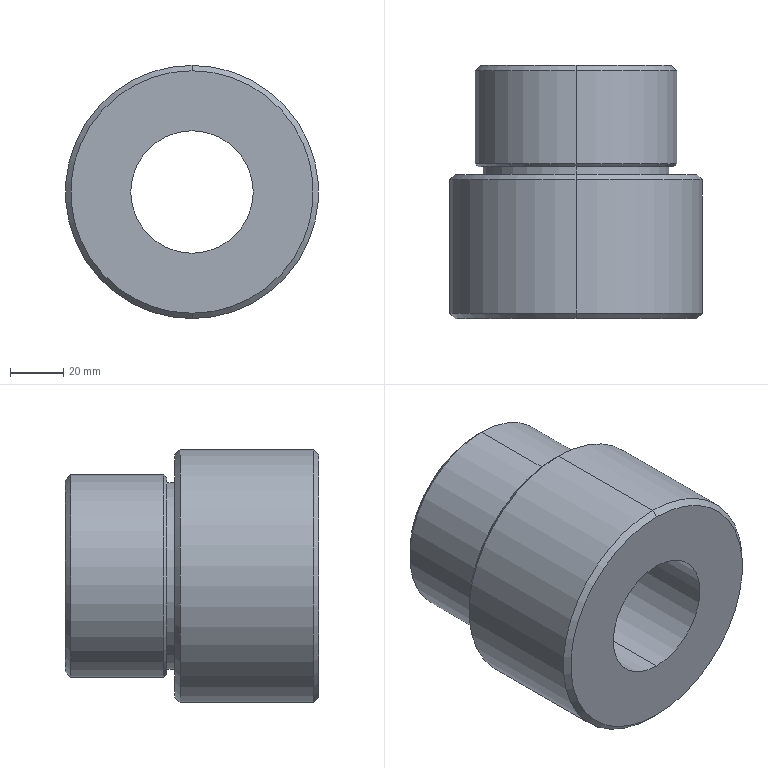Part | SolidWorks | features BaseBody 1 | 1 solid | 20 faces | box 95 x 95 x 95 mm | volume 407029 mm3 | cylinder 8 | cone 8 | plane 4 | commonest cylinder face diameters 46 x2 70 x2 76 x2 95 x2
STEP:
#1=CARTESIAN_POINT('',(0.,0.,-23.));
#2=VERTEX_POINT('',#1);
#3=CARTESIAN_POINT('',(0.,0.,23.));
#4=VERTEX_POINT('',#3);
#5=CARTESIAN_POINT('',(0.,0.,0.));
#6=DIRECTION('',(0.,1.,0.));
#7=DIRECTION('',(0.,0.,1.));
#8=AXIS2_PLACEMENT_3D('',#5,#6,#7);
#9=CIRCLE('',#8,23.);
#10=EDGE_CURVE('',#2,#4,#9,.T.);
#11=ORIENTED_EDGE('',*,*,#10,.F.);
#12=CARTESIAN_POINT('',(0.,95.,-23.));
#13=VERTEX_POINT('',#12);
#14=CARTESIAN_POINT('',(0.,95.,-23.));
#15=DIRECTION('',(0.,1.,0.));
#16=VECTOR('',#15,1000.);
#17=LINE('',#14,#16);
#18=EDGE_CURVE('',#2,#13,#17,.T.);
#19=ORIENTED_EDGE('',*,*,#18,.T.);
#20=CARTESIAN_POINT('',(0.,95.,23.));
#21=VERTEX_POINT('',#20);
#22=CARTESIAN_POINT('',(0.,95.,0.));
#23=DIRECTION('',(0.,1.,0.));
#24=DIRECTION('',(0.,0.,1.));
#25=AXIS2_PLACEMENT_3D('',#22,#23,#24);
#26=CIRCLE('',#25,23.);
#27=EDGE_CURVE('',#13,#21,#26,.T.);
#28=ORIENTED_EDGE('',*,*,#27,.T.);
#29=CARTESIAN_POINT('',(0.,95.,23.));
#30=DIRECTION('',(0.,1.,0.));
#31=VECTOR('',#30,1000.);
#32=LINE('',#29,#31);
#33=EDGE_CURVE('',#4,#21,#32,.T.);
#34=ORIENTED_EDGE('',*,*,#33,.F.);
#35=EDGE_LOOP('',(#11,#19,#28,#34));
#36=FACE_OUTER_BOUND('',#35,.T.);
#37=CARTESIAN_POINT('',(0.,95.,0.));
#38=DIRECTION('',(0.,1.,0.));
#39=DIRECTION('',(0.,0.,1.));
#40=AXIS2_PLACEMENT_3D('',#37,#38,#39);
#41=CYLINDRICAL_SURFACE('',#40,23.);
#42=ADVANCED_FACE('',(#36),#41,.F.);
#43=CARTESIAN_POINT('',(0.,93.,-38.));
#44=VERTEX_POINT('',#43);
#45=CARTESIAN_POINT('',(0.,93.,38.));
#46=VERTEX_POINT('',#45);
#47=CARTESIAN_POINT('',(0.,93.,0.));
#48=DIRECTION('',(0.,-1.,0.));
#49=DIRECTION('',(0.,0.,1.));
#50=AXIS2_PLACEMENT_3D('',#47,#48,#49);
#51=CIRCLE('',#50,38.);
#52=EDGE_CURVE('',#44,#46,#51,.T.);
#53=ORIENTED_EDGE('',*,*,#52,.T.);
#54=CARTESIAN_POINT('',(0.,58.083,38.));
#55=VERTEX_POINT('',#54);
#56=CARTESIAN_POINT('',(0.,95.,38.));
#57=DIRECTION('',(0.,-1.,0.));
#58=VECTOR('',#57,1000.);
#59=LINE('',#56,#58);
#60=EDGE_CURVE('',#46,#55,#59,.T.);
#61=ORIENTED_EDGE('',*,*,#60,.T.);
#62=CARTESIAN_POINT('',(0.,58.083,-38.));
#63=VERTEX_POINT('',#62);
#64=CARTESIAN_POINT('',(0.,58.083,0.));
#65=DIRECTION('',(0.,1.,0.));
#66=DIRECTION('',(0.,0.,1.));
#67=AXIS2_PLACEMENT_3D('',#64,#65,#66);
#68=CIRCLE('',#67,38.);
#69=EDGE_CURVE('',#55,#63,#68,.T.);
#70=ORIENTED_EDGE('',*,*,#69,.T.);
#71=CARTESIAN_POINT('',(0.,95.,-38.));
#72=DIRECTION('',(0.,-1.,0.));
#73=VECTOR('',#72,1000.);
#74=LINE('',#71,#73);
#75=EDGE_CURVE('',#44,#63,#74,.T.);
#76=ORIENTED_EDGE('',*,*,#75,.F.);
#77=EDGE_LOOP('',(#53,#61,#70,#76));
#78=FACE_OUTER_BOUND('',#77,.T.);
#79=CARTESIAN_POINT('',(0.,95.,0.));
#80=DIRECTION('',(0.,-1.,0.));
#81=DIRECTION('',(0.,0.,-1.));
#82=AXIS2_PLACEMENT_3D('',#79,#80,#81);
#83=CYLINDRICAL_SURFACE('',#82,38.);
#84=ADVANCED_FACE('',(#78),#83,.T.);
#85=CARTESIAN_POINT('',(0.,95.,36.));
#86=VERTEX_POINT('',#85);
#87=CARTESIAN_POINT('',(0.,95.,-36.));
#88=VERTEX_POINT('',#87);
#89=CARTESIAN_POINT('',(0.,95.,0.));
#90=DIRECTION('',(0.,1.,0.));
#91=DIRECTION('',(0.,0.,1.));
#92=AXIS2_PLACEMENT_3D('',#89,#90,#91);
#93=CIRCLE('',#92,36.);
#94=EDGE_CURVE('',#86,#88,#93,.T.);
#95=ORIENTED_EDGE('',*,*,#94,.F.);
#96=CARTESIAN_POINT('',(0.,95.,36.));
#97=DIRECTION('',(0.,-0.7071,0.7071));
#98=VECTOR('',#97,1000.);
#99=LINE('',#96,#98);
#100=EDGE_CURVE('',#86,#46,#99,.T.);
#101=ORIENTED_EDGE('',*,*,#100,.T.);
#102=ORIENTED_EDGE('',*,*,#52,.F.);
#103=CARTESIAN_POINT('',(0.,95.,-36.));
#104=DIRECTION('',(0.,-0.7071,-0.7071));
#105=VECTOR('',#104,1000.);
#106=LINE('',#103,#105);
#107=EDGE_CURVE('',#88,#44,#106,.T.);
#108=ORIENTED_EDGE('',*,*,#107,.F.);
#109=EDGE_LOOP('',(#95,#101,#102,#108));
#110=FACE_OUTER_BOUND('',#109,.T.);
#111=CARTESIAN_POINT('',(0.,95.,0.));
#112=DIRECTION('',(0.,-1.,0.));
#113=DIRECTION('',(0.,0.,-1.));
#114=AXIS2_PLACEMENT_3D('',#111,#112,#113);
#115=CONICAL_SURFACE('',#114,36.,0.7854);
#116=ADVANCED_FACE('',(#110),#115,.T.);
#117=CARTESIAN_POINT('',(0.,57.,36.917));
#118=VERTEX_POINT('',#117);
#119=CARTESIAN_POINT('',(0.,57.,-36.917));
#120=VERTEX_POINT('',#119);
#121=CARTESIAN_POINT('',(0.,57.,0.));
#122=DIRECTION('',(0.,1.,0.));
#123=DIRECTION('',(0.,0.,1.));
#124=AXIS2_PLACEMENT_3D('',#121,#122,#123);
#125=CIRCLE('',#124,36.917);
#126=EDGE_CURVE('',#118,#120,#125,.T.);
#127=ORIENTED_EDGE('',*,*,#126,.T.);
#128=CARTESIAN_POINT('',(0.,57.,-36.917));
#129=DIRECTION('',(0.,0.7071,-0.7071));
#130=VECTOR('',#129,1000.);
#131=LINE('',#128,#130);
#132=EDGE_CURVE('',#120,#63,#131,.T.);
#133=ORIENTED_EDGE('',*,*,#132,.T.);
#134=ORIENTED_EDGE('',*,*,#69,.F.);
#135=CARTESIAN_POINT('',(0.,57.,36.917));
#136=DIRECTION('',(0.,0.7071,0.7071));
#137=VECTOR('',#136,1000.);
#138=LINE('',#135,#137);
#139=EDGE_CURVE('',#118,#55,#138,.T.);
#140=ORIENTED_EDGE('',*,*,#139,.F.);
#141=EDGE_LOOP('',(#127,#133,#134,#140));
#142=FACE_OUTER_BOUND('',#141,.T.);
#143=CARTESIAN_POINT('',(0.,57.,0.));
#144=DIRECTION('',(0.,1.,0.));
#145=DIRECTION('',(0.,0.,1.));
#146=AXIS2_PLACEMENT_3D('',#143,#144,#145);
#147=CONICAL_SURFACE('',#146,36.917,0.7854);
#148=ADVANCED_FACE('',(#142),#147,.T.);
#149=CARTESIAN_POINT('',(0.,54.,45.5));
#150=VERTEX_POINT('',#149);
#151=CARTESIAN_POINT('',(0.,54.,-45.5));
#152=VERTEX_POINT('',#151);
#153=CARTESIAN_POINT('',(0.,54.,0.));
#154=DIRECTION('',(0.,1.,0.));
#155=DIRECTION('',(0.,0.,1.));
#156=AXIS2_PLACEMENT_3D('',#153,#154,#155);
#157=CIRCLE('',#156,45.5);
#158=EDGE_CURVE('',#150,#152,#157,.T.);
#159=ORIENTED_EDGE('',*,*,#158,.F.);
#160=CARTESIAN_POINT('',(0.,52.,47.5));
#161=VERTEX_POINT('',#160);
#162=CARTESIAN_POINT('',(0.,54.,45.5));
#163=DIRECTION('',(0.,-0.7071,0.7071));
#164=VECTOR('',#163,1000.);
#165=LINE('',#162,#164);
#166=EDGE_CURVE('',#150,#161,#165,.T.);
#167=ORIENTED_EDGE('',*,*,#166,.T.);
#168=CARTESIAN_POINT('',(0.,52.,-47.5));
#169=VERTEX_POINT('',#168);
#170=CARTESIAN_POINT('',(0.,52.,0.));
#171=DIRECTION('',(0.,-1.,0.));
#172=DIRECTION('',(0.,0.,1.));
#173=AXIS2_PLACEMENT_3D('',#170,#171,#172);
#174=CIRCLE('',#173,47.5);
#175=EDGE_CURVE('',#169,#161,#174,.T.);
#176=ORIENTED_EDGE('',*,*,#175,.F.);
#177=CARTESIAN_POINT('',(0.,54.,-45.5));
#178=DIRECTION('',(0.,-0.7071,-0.7071));
#179=VECTOR('',#178,1000.);
#180=LINE('',#177,#179);
#181=EDGE_CURVE('',#152,#169,#180,.T.);
#182=ORIENTED_EDGE('',*,*,#181,.F.);
#183=EDGE_LOOP('',(#159,#167,#176,#182));
#184=FACE_OUTER_BOUND('',#183,.T.);
#185=CARTESIAN_POINT('',(0.,54.,0.));
#186=DIRECTION('',(0.,-1.,0.));
#187=DIRECTION('',(0.,0.,-1.));
#188=AXIS2_PLACEMENT_3D('',#185,#186,#187);
#189=CONICAL_SURFACE('',#188,45.5,0.7854);
#190=ADVANCED_FACE('',(#184),#189,.T.);
#191=CARTESIAN_POINT('',(0.,0.,-45.5));
#192=VERTEX_POINT('',#191);
#193=CARTESIAN_POINT('',(0.,0.,45.5));
#194=VERTEX_POINT('',#193);
#195=CARTESIAN_POINT('',(0.,0.,0.));
#196=DIRECTION('',(0.,-1.,0.));
#197=DIRECTION('',(0.,0.,1.));
#198=AXIS2_PLACEMENT_3D('',#195,#196,#197);
#199=CIRCLE('',#198,45.5);
#200=EDGE_CURVE('',#192,#194,#199,.T.);
#201=ORIENTED_EDGE('',*,*,#200,.F.);
#202=CARTESIAN_POINT('',(0.,2.,-47.5));
#203=VERTEX_POINT('',#202);
#204=CARTESIAN_POINT('',(0.,2.,-47.5));
#205=DIRECTION('',(0.,0.7071,-0.7071));
#206=VECTOR('',#205,1000.);
#207=LINE('',#204,#206);
#208=EDGE_CURVE('',#192,#203,#207,.T.);
#209=ORIENTED_EDGE('',*,*,#208,.T.);
#210=CARTESIAN_POINT('',(0.,2.,47.5));
#211=VERTEX_POINT('',#210);
#212=CARTESIAN_POINT('',(0.,2.,0.));
#213=DIRECTION('',(0.,1.,0.));
#214=DIRECTION('',(0.,0.,1.));
#215=AXIS2_PLACEMENT_3D('',#212,#213,#214);
#216=CIRCLE('',#215,47.5);
#217=EDGE_CURVE('',#211,#203,#216,.T.);
#218=ORIENTED_EDGE('',*,*,#217,.F.);
#219=CARTESIAN_POINT('',(0.,2.,47.5));
#220=DIRECTION('',(0.,0.7071,0.7071));
#221=VECTOR('',#220,1000.);
#222=LINE('',#219,#221);
#223=EDGE_CURVE('',#194,#211,#222,.T.);
#224=ORIENTED_EDGE('',*,*,#223,.F.);
#225=EDGE_LOOP('',(#201,#209,#218,#224));
#226=FACE_OUTER_BOUND('',#225,.T.);
#227=CARTESIAN_POINT('',(0.,2.,0.));
#228=DIRECTION('',(0.,1.,0.));
#229=DIRECTION('',(0.,0.,1.));
#230=AXIS2_PLACEMENT_3D('',#227,#228,#229);
#231=CONICAL_SURFACE('',#230,47.5,0.7854);
#232=ADVANCED_FACE('',(#226),#231,.T.);
#233=CARTESIAN_POINT('',(0.,57.,35.));
#234=VERTEX_POINT('',#233);
#235=CARTESIAN_POINT('',(0.,57.,-35.));
#236=VERTEX_POINT('',#235);
#237=CARTESIAN_POINT('',(0.,57.,0.));
#238=DIRECTION('',(0.,1.,0.));
#239=DIRECTION('',(0.,0.,1.));
#240=AXIS2_PLACEMENT_3D('',#237,#238,#239);
#241=CIRCLE('',#240,35.);
#242=EDGE_CURVE('',#234,#236,#241,.T.);
#243=ORIENTED_EDGE('',*,*,#242,.F.);
#244=CARTESIAN_POINT('',(0.,54.,35.));
#245=VERTEX_POINT('',#244);
#246=CARTESIAN_POINT('',(0.,57.,35.));
#247=DIRECTION('',(0.,-1.,0.));
#248=VECTOR('',#247,1000.);
#249=LINE('',#246,#248);
#250=EDGE_CURVE('',#234,#245,#249,.T.);
#251=ORIENTED_EDGE('',*,*,#250,.T.);
#252=CARTESIAN_POINT('',(0.,54.,-35.));
#253=VERTEX_POINT('',#252);
#254=CARTESIAN_POINT('',(0.,54.,0.));
#255=DIRECTION('',(0.,1.,0.));
#256=DIRECTION('',(0.,0.,1.));
#257=AXIS2_PLACEMENT_3D('',#254,#255,#256);
#258=CIRCLE('',#257,35.);
#259=EDGE_CURVE('',#245,#253,#258,.T.);
#260=ORIENTED_EDGE('',*,*,#259,.T.);
#261=CARTESIAN_POINT('',(0.,57.,-35.));
#262=DIRECTION('',(0.,-1.,0.));
#263=VECTOR('',#262,1000.);
#264=LINE('',#261,#263);
#265=EDGE_CURVE('',#236,#253,#264,.T.);
#266=ORIENTED_EDGE('',*,*,#265,.F.);
#267=EDGE_LOOP('',(#243,#251,#260,#266));
#268=FACE_OUTER_BOUND('',#267,.T.);
#269=CARTESIAN_POINT('',(0.,57.,0.));
#270=DIRECTION('',(0.,-1.,0.));
#271=DIRECTION('',(0.,0.,-1.));
#272=AXIS2_PLACEMENT_3D('',#269,#270,#271);
#273=CYLINDRICAL_SURFACE('',#272,35.);
#274=ADVANCED_FACE('',(#268),#273,.T.);
#275=ORIENTED_EDGE('',*,*,#175,.T.);
#276=CARTESIAN_POINT('',(0.,54.,47.5));
#277=DIRECTION('',(0.,-1.,0.));
#278=VECTOR('',#277,1000.);
#279=LINE('',#276,#278);
#280=EDGE_CURVE('',#161,#211,#279,.T.);
#281=ORIENTED_EDGE('',*,*,#280,.T.);
#282=ORIENTED_EDGE('',*,*,#217,.T.);
#283=CARTESIAN_POINT('',(0.,54.,-47.5));
#284=DIRECTION('',(0.,-1.,0.));
#285=VECTOR('',#284,1000.);
#286=LINE('',#283,#285);
#287=EDGE_CURVE('',#169,#203,#286,.T.);
#288=ORIENTED_EDGE('',*,*,#287,.F.);
#289=EDGE_LOOP('',(#275,#281,#282,#288));
#290=FACE_OUTER_BOUND('',#289,.T.);
#291=CARTESIAN_POINT('',(0.,54.,0.));
#292=DIRECTION('',(0.,-1.,0.));
#293=DIRECTION('',(0.,0.,-1.));
#294=AXIS2_PLACEMENT_3D('',#291,#292,#293);
#295=CYLINDRICAL_SURFACE('',#294,47.5);
#296=ADVANCED_FACE('',(#290),#295,.T.);
#297=CARTESIAN_POINT('',(0.,57.,0.));
#298=DIRECTION('',(0.,1.,0.));
#299=DIRECTION('',(0.,0.,1.));
#300=AXIS2_PLACEMENT_3D('',#297,#298,#299);
#301=CIRCLE('',#300,35.);
#302=EDGE_CURVE('',#236,#234,#301,.T.);
#303=ORIENTED_EDGE('',*,*,#302,.T.);
#304=ORIENTED_EDGE('',*,*,#242,.T.);
#305=EDGE_LOOP('',(#303,#304));
#306=FACE_BOUND('',#305,.T.);
#307=ORIENTED_EDGE('',*,*,#126,.F.);
#308=CARTESIAN_POINT('',(0.,57.,0.));
#309=DIRECTION('',(0.,1.,0.));
#310=DIRECTION('',(0.,0.,1.));
#311=AXIS2_PLACEMENT_3D('',#308,#309,#310);
#312=CIRCLE('',#311,36.917);
#313=EDGE_CURVE('',#120,#118,#312,.T.);
#314=ORIENTED_EDGE('',*,*,#313,.F.);
#315=EDGE_LOOP('',(#307,#314));
#316=FACE_OUTER_BOUND('',#315,.T.);
#317=CARTESIAN_POINT('',(0.,57.,0.));
#318=DIRECTION('',(0.,1.,0.));
#319=DIRECTION('',(0.,0.,1.));
#320=AXIS2_PLACEMENT_3D('',#317,#318,#319);
#321=PLANE('',#320);
#322=ADVANCED_FACE('',(#306,#316),#321,.F.);
#323=ORIENTED_EDGE('',*,*,#280,.F.);
#324=CARTESIAN_POINT('',(0.,52.,0.));
#325=DIRECTION('',(0.,-1.,0.));
#326=DIRECTION('',(0.,0.,1.));
#327=AXIS2_PLACEMENT_3D('',#324,#325,#326);
#328=CIRCLE('',#327,47.5);
#329=EDGE_CURVE('',#161,#169,#328,.T.);
#330=ORIENTED_EDGE('',*,*,#329,.T.);
#331=ORIENTED_EDGE('',*,*,#287,.T.);
#332=CARTESIAN_POINT('',(0.,2.,0.));
#333=DIRECTION('',(0.,1.,0.));
#334=DIRECTION('',(0.,0.,1.));
#335=AXIS2_PLACEMENT_3D('',#332,#333,#334);
#336=CIRCLE('',#335,47.5);
#337=EDGE_CURVE('',#203,#211,#336,.T.);
#338=ORIENTED_EDGE('',*,*,#337,.T.);
#339=EDGE_LOOP('',(#323,#330,#331,#338));
#340=FACE_OUTER_BOUND('',#339,.T.);
#341=CARTESIAN_POINT('',(0.,54.,0.));
#342=DIRECTION('',(0.,-1.,0.));
#343=DIRECTION('',(0.,0.,-1.));
#344=AXIS2_PLACEMENT_3D('',#341,#342,#343);
#345=CYLINDRICAL_SURFACE('',#344,47.5);
#346=ADVANCED_FACE('',(#340),#345,.T.);
#347=CARTESIAN_POINT('',(0.,54.,0.));
#348=DIRECTION('',(0.,1.,0.));
#349=DIRECTION('',(0.,0.,1.));
#350=AXIS2_PLACEMENT_3D('',#347,#348,#349);
#351=CIRCLE('',#350,45.5);
#352=EDGE_CURVE('',#152,#150,#351,.T.);
#353=ORIENTED_EDGE('',*,*,#352,.T.);
#354=ORIENTED_EDGE('',*,*,#158,.T.);
#355=EDGE_LOOP('',(#353,#354));
#356=FACE_OUTER_BOUND('',#355,.T.);
#357=CARTESIAN_POINT('',(0.,54.,0.));
#358=DIRECTION('',(0.,1.,0.));
#359=DIRECTION('',(0.,0.,1.));
#360=AXIS2_PLACEMENT_3D('',#357,#358,#359);
#361=CIRCLE('',#360,35.);
#362=EDGE_CURVE('',#253,#245,#361,.T.);
#363=ORIENTED_EDGE('',*,*,#362,.F.);
#364=ORIENTED_EDGE('',*,*,#259,.F.);
#365=EDGE_LOOP('',(#363,#364));
#366=FACE_BOUND('',#365,.T.);
#367=CARTESIAN_POINT('',(0.,54.,0.));
#368=DIRECTION('',(0.,1.,0.));
#369=DIRECTION('',(0.,0.,1.));
#370=AXIS2_PLACEMENT_3D('',#367,#368,#369);
#371=PLANE('',#370);
#372=ADVANCED_FACE('',(#356,#366),#371,.T.);
#373=CARTESIAN_POINT('',(0.,0.,0.));
#374=DIRECTION('',(0.,1.,0.));
#375=DIRECTION('',(0.,0.,1.));
#376=AXIS2_PLACEMENT_3D('',#373,#374,#375);
#377=CIRCLE('',#376,23.);
#378=EDGE_CURVE('',#4,#2,#377,.T.);
#379=ORIENTED_EDGE('',*,*,#378,.T.);
#380=ORIENTED_EDGE('',*,*,#10,.T.);
#381=EDGE_LOOP('',(#379,#380));
#382=FACE_BOUND('',#381,.T.);
#383=CARTESIAN_POINT('',(0.,0.,0.));
#384=DIRECTION('',(0.,-1.,0.));
#385=DIRECTION('',(0.,0.,1.));
#386=AXIS2_PLACEMENT_3D('',#383,#384,#385);
#387=CIRCLE('',#386,45.5);
#388=EDGE_CURVE('',#194,#192,#387,.T.);
#389=ORIENTED_EDGE('',*,*,#388,.T.);
#390=ORIENTED_EDGE('',*,*,#200,.T.);
#391=EDGE_LOOP('',(#389,#390));
#392=FACE_OUTER_BOUND('',#391,.T.);
#393=CARTESIAN_POINT('',(0.,0.,0.));
#394=DIRECTION('',(0.,1.,0.));
#395=DIRECTION('',(0.,0.,1.));
#396=AXIS2_PLACEMENT_3D('',#393,#394,#395);
#397=PLANE('',#396);
#398=ADVANCED_FACE('',(#382,#392),#397,.F.);
#399=ORIENTED_EDGE('',*,*,#250,.F.);
#400=ORIENTED_EDGE('',*,*,#302,.F.);
#401=ORIENTED_EDGE('',*,*,#265,.T.);
#402=ORIENTED_EDGE('',*,*,#362,.T.);
#403=EDGE_LOOP('',(#399,#400,#401,#402));
#404=FACE_OUTER_BOUND('',#403,.T.);
#405=CARTESIAN_POINT('',(0.,57.,0.));
#406=DIRECTION('',(0.,-1.,0.));
#407=DIRECTION('',(0.,0.,-1.));
#408=AXIS2_PLACEMENT_3D('',#405,#406,#407);
#409=CYLINDRICAL_SURFACE('',#408,35.);
#410=ADVANCED_FACE('',(#404),#409,.T.);
#411=ORIENTED_EDGE('',*,*,#208,.F.);
#412=ORIENTED_EDGE('',*,*,#388,.F.);
#413=ORIENTED_EDGE('',*,*,#223,.T.);
#414=ORIENTED_EDGE('',*,*,#337,.F.);
#415=EDGE_LOOP('',(#411,#412,#413,#414));
#416=FACE_OUTER_BOUND('',#415,.T.);
#417=CARTESIAN_POINT('',(0.,2.,0.));
#418=DIRECTION('',(0.,1.,0.));
#419=DIRECTION('',(0.,0.,1.));
#420=AXIS2_PLACEMENT_3D('',#417,#418,#419);
#421=CONICAL_SURFACE('',#420,47.5,0.7854);
#422=ADVANCED_FACE('',(#416),#421,.T.);
#423=ORIENTED_EDGE('',*,*,#166,.F.);
#424=ORIENTED_EDGE('',*,*,#352,.F.);
#425=ORIENTED_EDGE('',*,*,#181,.T.);
#426=ORIENTED_EDGE('',*,*,#329,.F.);
#427=EDGE_LOOP('',(#423,#424,#425,#426));
#428=FACE_OUTER_BOUND('',#427,.T.);
#429=CARTESIAN_POINT('',(0.,54.,0.));
#430=DIRECTION('',(0.,-1.,0.));
#431=DIRECTION('',(0.,0.,-1.));
#432=AXIS2_PLACEMENT_3D('',#429,#430,#431);
#433=CONICAL_SURFACE('',#432,45.5,0.7854);
#434=ADVANCED_FACE('',(#428),#433,.T.);
#435=ORIENTED_EDGE('',*,*,#132,.F.);
#436=ORIENTED_EDGE('',*,*,#313,.T.);
#437=ORIENTED_EDGE('',*,*,#139,.T.);
#438=CARTESIAN_POINT('',(0.,58.083,0.));
#439=DIRECTION('',(0.,1.,0.));
#440=DIRECTION('',(0.,0.,1.));
#441=AXIS2_PLACEMENT_3D('',#438,#439,#440);
#442=CIRCLE('',#441,38.);
#443=EDGE_CURVE('',#63,#55,#442,.T.);
#444=ORIENTED_EDGE('',*,*,#443,.F.);
#445=EDGE_LOOP('',(#435,#436,#437,#444));
#446=FACE_OUTER_BOUND('',#445,.T.);
#447=CARTESIAN_POINT('',(0.,57.,0.));
#448=DIRECTION('',(0.,1.,0.));
#449=DIRECTION('',(0.,0.,1.));
#450=AXIS2_PLACEMENT_3D('',#447,#448,#449);
#451=CONICAL_SURFACE('',#450,36.917,0.7854);
#452=ADVANCED_FACE('',(#446),#451,.T.);
#453=CARTESIAN_POINT('',(0.,95.,0.));
#454=DIRECTION('',(0.,1.,0.));
#455=DIRECTION('',(0.,0.,1.));
#456=AXIS2_PLACEMENT_3D('',#453,#454,#455);
#457=CIRCLE('',#456,23.);
#458=EDGE_CURVE('',#21,#13,#457,.T.);
#459=ORIENTED_EDGE('',*,*,#458,.F.);
#460=ORIENTED_EDGE('',*,*,#27,.F.);
#461=EDGE_LOOP('',(#459,#460));
#462=FACE_BOUND('',#461,.T.);
#463=CARTESIAN_POINT('',(0.,95.,0.));
#464=DIRECTION('',(0.,1.,0.));
#465=DIRECTION('',(0.,0.,1.));
#466=AXIS2_PLACEMENT_3D('',#463,#464,#465);
#467=CIRCLE('',#466,36.);
#468=EDGE_CURVE('',#88,#86,#467,.T.);
#469=ORIENTED_EDGE('',*,*,#468,.T.);
#470=ORIENTED_EDGE('',*,*,#94,.T.);
#471=EDGE_LOOP('',(#469,#470));
#472=FACE_OUTER_BOUND('',#471,.T.);
#473=CARTESIAN_POINT('',(0.,95.,0.));
#474=DIRECTION('',(0.,1.,0.));
#475=DIRECTION('',(0.,0.,1.));
#476=AXIS2_PLACEMENT_3D('',#473,#474,#475);
#477=PLANE('',#476);
#478=ADVANCED_FACE('',(#462,#472),#477,.T.);
#479=ORIENTED_EDGE('',*,*,#100,.F.);
#480=ORIENTED_EDGE('',*,*,#468,.F.);
#481=ORIENTED_EDGE('',*,*,#107,.T.);
#482=CARTESIAN_POINT('',(0.,93.,0.));
#483=DIRECTION('',(0.,-1.,0.));
#484=DIRECTION('',(0.,0.,1.));
#485=AXIS2_PLACEMENT_3D('',#482,#483,#484);
#486=CIRCLE('',#485,38.);
#487=EDGE_CURVE('',#46,#44,#486,.T.);
#488=ORIENTED_EDGE('',*,*,#487,.F.);
#489=EDGE_LOOP('',(#479,#480,#481,#488));
#490=FACE_OUTER_BOUND('',#489,.T.);
#491=CARTESIAN_POINT('',(0.,95.,0.));
#492=DIRECTION('',(0.,-1.,0.));
#493=DIRECTION('',(0.,0.,-1.));
#494=AXIS2_PLACEMENT_3D('',#491,#492,#493);
#495=CONICAL_SURFACE('',#494,36.,0.7854);
#496=ADVANCED_FACE('',(#490),#495,.T.);
#497=ORIENTED_EDGE('',*,*,#60,.F.);
#498=ORIENTED_EDGE('',*,*,#487,.T.);
#499=ORIENTED_EDGE('',*,*,#75,.T.);
#500=ORIENTED_EDGE('',*,*,#443,.T.);
#501=EDGE_LOOP('',(#497,#498,#499,#500));
#502=FACE_OUTER_BOUND('',#501,.T.);
#503=CARTESIAN_POINT('',(0.,95.,0.));
#504=DIRECTION('',(0.,-1.,0.));
#505=DIRECTION('',(0.,0.,-1.));
#506=AXIS2_PLACEMENT_3D('',#503,#504,#505);
#507=CYLINDRICAL_SURFACE('',#506,38.);
#508=ADVANCED_FACE('',(#502),#507,.T.);
#509=ORIENTED_EDGE('',*,*,#18,.F.);
#510=ORIENTED_EDGE('',*,*,#378,.F.);
#511=ORIENTED_EDGE('',*,*,#33,.T.);
#512=ORIENTED_EDGE('',*,*,#458,.T.);
#513=EDGE_LOOP('',(#509,#510,#511,#512));
#514=FACE_OUTER_BOUND('',#513,.T.);
#515=CARTESIAN_POINT('',(0.,95.,0.));
#516=DIRECTION('',(0.,1.,0.));
#517=DIRECTION('',(0.,0.,1.));
#518=AXIS2_PLACEMENT_3D('',#515,#516,#517);
#519=CYLINDRICAL_SURFACE('',#518,23.);
#520=ADVANCED_FACE('',(#514),#519,.F.);
#521=CLOSED_SHELL('',(#42,#84,#116,#148,#190,#232,#274,#296,#322,#346,#372,#398,#410,#422,#434,#452,#478,#496,#508,#520));
#522=MANIFOLD_SOLID_BREP('',#521);
#523=CARTESIAN_POINT('',(0.,0.,0.));
#524=DIRECTION('',(0.,0.,1.));
#525=DIRECTION('',(1.,0.,0.));
#526=AXIS2_PLACEMENT_3D('',#523,#524,#525);
#527=(LENGTH_UNIT()NAMED_UNIT(*)SI_UNIT(.MILLI.,.METRE.));
#528=UNCERTAINTY_MEASURE_WITH_UNIT(LENGTH_MEASURE(0.00001),#527,'','');
#529=(NAMED_UNIT(*)PLANE_ANGLE_UNIT()SI_UNIT($,.RADIAN.));
#530=(NAMED_UNIT(*)SI_UNIT($,.STERADIAN.)SOLID_ANGLE_UNIT());
#531=(GEOMETRIC_REPRESENTATION_CONTEXT(3)GLOBAL_UNCERTAINTY_ASSIGNED_CONTEXT((#528))GLOBAL_UNIT_ASSIGNED_CONTEXT((#527,#529,#530))REPRESENTATION_CONTEXT('',''));
#532=ADVANCED_BREP_SHAPE_REPRESENTATION('',(#522,#526),#531);